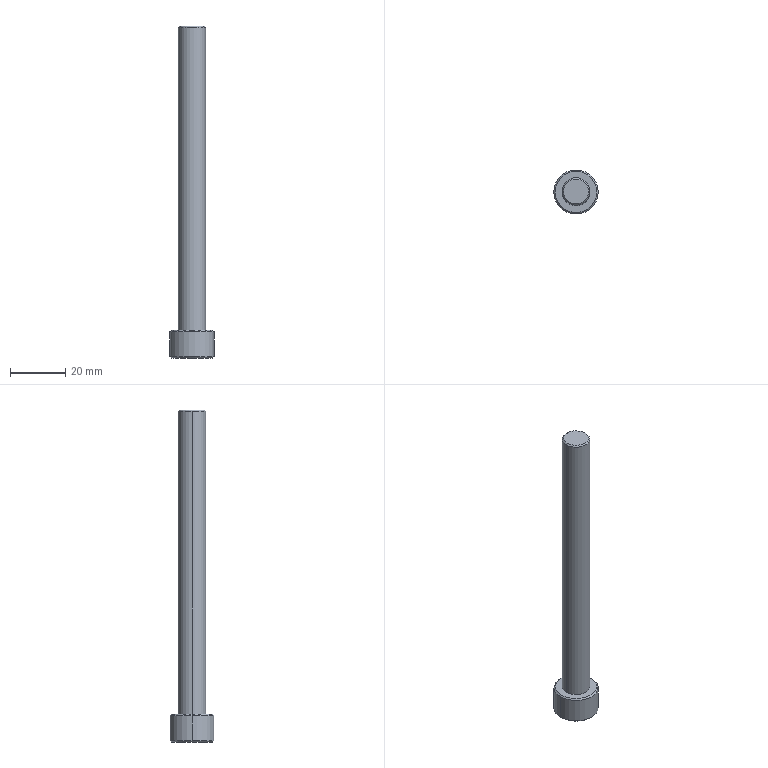Part | SolidWorks | features Chamfer 1, Extrusion 1, ICE 1 | 1 solid | 13 faces | box 16 x 16 x 120 mm | volume 10634 mm3 | cone 6 | cylinder 4 | plane 3 | commonest cylinder face diameters 10 x2 16 x2
STEP:
#1=CARTESIAN_POINT('',(7.5,0.,0.));
#2=VERTEX_POINT('',#1);
#3=CARTESIAN_POINT('',(-7.5,0.,0.));
#4=VERTEX_POINT('',#3);
#5=CARTESIAN_POINT('',(0.,0.,0.));
#6=DIRECTION('',(0.,0.,1.));
#7=DIRECTION('',(-1.,0.,0.));
#8=AXIS2_PLACEMENT_3D('',#5,#6,#7);
#9=CIRCLE('',#8,7.5);
#10=EDGE_CURVE('',#2,#4,#9,.T.);
#11=ORIENTED_EDGE('',*,*,#10,.F.);
#12=CARTESIAN_POINT('',(8.,0.,-0.5));
#13=VERTEX_POINT('',#12);
#14=CARTESIAN_POINT('',(8.,0.,-0.5));
#15=DIRECTION('',(0.7071,0.,-0.7071));
#16=VECTOR('',#15,1000.);
#17=LINE('',#14,#16);
#18=EDGE_CURVE('',#2,#13,#17,.T.);
#19=ORIENTED_EDGE('',*,*,#18,.T.);
#20=CARTESIAN_POINT('',(-8.,0.,-0.5));
#21=VERTEX_POINT('',#20);
#22=CARTESIAN_POINT('',(0.,0.,-0.5));
#23=DIRECTION('',(0.,0.,-1.));
#24=DIRECTION('',(-1.,0.,0.));
#25=AXIS2_PLACEMENT_3D('',#22,#23,#24);
#26=CIRCLE('',#25,8.);
#27=EDGE_CURVE('',#21,#13,#26,.T.);
#28=ORIENTED_EDGE('',*,*,#27,.F.);
#29=CARTESIAN_POINT('',(-8.,0.,-0.5));
#30=DIRECTION('',(-0.7071,0.,-0.7071));
#31=VECTOR('',#30,1000.);
#32=LINE('',#29,#31);
#33=EDGE_CURVE('',#4,#21,#32,.T.);
#34=ORIENTED_EDGE('',*,*,#33,.F.);
#35=EDGE_LOOP('',(#11,#19,#28,#34));
#36=FACE_OUTER_BOUND('',#35,.T.);
#37=CARTESIAN_POINT('',(0.,0.,-0.5));
#38=DIRECTION('',(0.,0.,-1.));
#39=DIRECTION('',(-1.,0.,0.));
#40=AXIS2_PLACEMENT_3D('',#37,#38,#39);
#41=CONICAL_SURFACE('',#40,8.,0.7854);
#42=ADVANCED_FACE('',(#36),#41,.T.);
#43=CARTESIAN_POINT('',(-7.5,0.,-10.));
#44=VERTEX_POINT('',#43);
#45=CARTESIAN_POINT('',(7.5,0.,-10.));
#46=VERTEX_POINT('',#45);
#47=CARTESIAN_POINT('',(0.,0.,-10.));
#48=DIRECTION('',(0.,0.,-1.));
#49=DIRECTION('',(-1.,0.,0.));
#50=AXIS2_PLACEMENT_3D('',#47,#48,#49);
#51=CIRCLE('',#50,7.5);
#52=EDGE_CURVE('',#44,#46,#51,.T.);
#53=ORIENTED_EDGE('',*,*,#52,.F.);
#54=CARTESIAN_POINT('',(-8.,0.,-9.5));
#55=VERTEX_POINT('',#54);
#56=CARTESIAN_POINT('',(-7.5,0.,-10.));
#57=DIRECTION('',(-0.7071,0.,0.7071));
#58=VECTOR('',#57,1000.);
#59=LINE('',#56,#58);
#60=EDGE_CURVE('',#44,#55,#59,.T.);
#61=ORIENTED_EDGE('',*,*,#60,.T.);
#62=CARTESIAN_POINT('',(8.,0.,-9.5));
#63=VERTEX_POINT('',#62);
#64=CARTESIAN_POINT('',(0.,0.,-9.5));
#65=DIRECTION('',(0.,0.,1.));
#66=DIRECTION('',(-1.,0.,0.));
#67=AXIS2_PLACEMENT_3D('',#64,#65,#66);
#68=CIRCLE('',#67,8.);
#69=EDGE_CURVE('',#63,#55,#68,.T.);
#70=ORIENTED_EDGE('',*,*,#69,.F.);
#71=CARTESIAN_POINT('',(7.5,0.,-10.));
#72=DIRECTION('',(0.7071,0.,0.7071));
#73=VECTOR('',#72,1000.);
#74=LINE('',#71,#73);
#75=EDGE_CURVE('',#46,#63,#74,.T.);
#76=ORIENTED_EDGE('',*,*,#75,.F.);
#77=EDGE_LOOP('',(#53,#61,#70,#76));
#78=FACE_OUTER_BOUND('',#77,.T.);
#79=CARTESIAN_POINT('',(0.,0.,-10.));
#80=DIRECTION('',(0.,0.,1.));
#81=DIRECTION('',(1.,0.,0.));
#82=AXIS2_PLACEMENT_3D('',#79,#80,#81);
#83=CONICAL_SURFACE('',#82,7.5,0.7854);
#84=ADVANCED_FACE('',(#78),#83,.T.);
#85=CARTESIAN_POINT('',(4.5,0.,110.));
#86=VERTEX_POINT('',#85);
#87=CARTESIAN_POINT('',(-4.5,0.,110.));
#88=VERTEX_POINT('',#87);
#89=CARTESIAN_POINT('',(0.,0.,110.));
#90=DIRECTION('',(0.,0.,1.));
#91=DIRECTION('',(1.,0.,0.));
#92=AXIS2_PLACEMENT_3D('',#89,#90,#91);
#93=CIRCLE('',#92,4.5);
#94=EDGE_CURVE('',#86,#88,#93,.T.);
#95=ORIENTED_EDGE('',*,*,#94,.F.);
#96=CARTESIAN_POINT('',(5.,0.,109.5));
#97=VERTEX_POINT('',#96);
#98=CARTESIAN_POINT('',(4.5,0.,110.));
#99=DIRECTION('',(0.7071,0.,-0.7071));
#100=VECTOR('',#99,1000.);
#101=LINE('',#98,#100);
#102=EDGE_CURVE('',#86,#97,#101,.T.);
#103=ORIENTED_EDGE('',*,*,#102,.T.);
#104=CARTESIAN_POINT('',(-5.,0.,109.5));
#105=VERTEX_POINT('',#104);
#106=CARTESIAN_POINT('',(0.,0.,109.5));
#107=DIRECTION('',(0.,0.,-1.));
#108=DIRECTION('',(1.,0.,0.));
#109=AXIS2_PLACEMENT_3D('',#106,#107,#108);
#110=CIRCLE('',#109,5.);
#111=EDGE_CURVE('',#105,#97,#110,.T.);
#112=ORIENTED_EDGE('',*,*,#111,.F.);
#113=CARTESIAN_POINT('',(-4.5,0.,110.));
#114=DIRECTION('',(-0.7071,0.,-0.7071));
#115=VECTOR('',#114,1000.);
#116=LINE('',#113,#115);
#117=EDGE_CURVE('',#88,#105,#116,.T.);
#118=ORIENTED_EDGE('',*,*,#117,.F.);
#119=EDGE_LOOP('',(#95,#103,#112,#118));
#120=FACE_OUTER_BOUND('',#119,.T.);
#121=CARTESIAN_POINT('',(0.,0.,110.));
#122=DIRECTION('',(0.,0.,-1.));
#123=DIRECTION('',(-1.,0.,0.));
#124=AXIS2_PLACEMENT_3D('',#121,#122,#123);
#125=CONICAL_SURFACE('',#124,4.5,0.7854);
#126=ADVANCED_FACE('',(#120),#125,.T.);
#127=ORIENTED_EDGE('',*,*,#69,.T.);
#128=CARTESIAN_POINT('',(-8.,0.,-10.));
#129=DIRECTION('',(0.,0.,1.));
#130=VECTOR('',#129,1000.);
#131=LINE('',#128,#130);
#132=EDGE_CURVE('',#55,#21,#131,.T.);
#133=ORIENTED_EDGE('',*,*,#132,.T.);
#134=ORIENTED_EDGE('',*,*,#27,.T.);
#135=CARTESIAN_POINT('',(8.,0.,-10.));
#136=DIRECTION('',(0.,0.,1.));
#137=VECTOR('',#136,1000.);
#138=LINE('',#135,#137);
#139=EDGE_CURVE('',#63,#13,#138,.T.);
#140=ORIENTED_EDGE('',*,*,#139,.F.);
#141=EDGE_LOOP('',(#127,#133,#134,#140));
#142=FACE_OUTER_BOUND('',#141,.T.);
#143=CARTESIAN_POINT('',(0.,0.,-10.));
#144=DIRECTION('',(0.,0.,1.));
#145=DIRECTION('',(1.,0.,0.));
#146=AXIS2_PLACEMENT_3D('',#143,#144,#145);
#147=CYLINDRICAL_SURFACE('',#146,8.);
#148=ADVANCED_FACE('',(#142),#147,.T.);
#149=ORIENTED_EDGE('',*,*,#111,.T.);
#150=CARTESIAN_POINT('',(5.,0.,0.));
#151=VERTEX_POINT('',#150);
#152=CARTESIAN_POINT('',(5.,0.,110.));
#153=DIRECTION('',(0.,0.,-1.));
#154=VECTOR('',#153,1000.);
#155=LINE('',#152,#154);
#156=EDGE_CURVE('',#97,#151,#155,.T.);
#157=ORIENTED_EDGE('',*,*,#156,.T.);
#158=CARTESIAN_POINT('',(-5.,0.,0.));
#159=VERTEX_POINT('',#158);
#160=CARTESIAN_POINT('',(0.,0.,0.));
#161=DIRECTION('',(0.,0.,1.));
#162=DIRECTION('',(1.,0.,0.));
#163=AXIS2_PLACEMENT_3D('',#160,#161,#162);
#164=CIRCLE('',#163,5.);
#165=EDGE_CURVE('',#151,#159,#164,.T.);
#166=ORIENTED_EDGE('',*,*,#165,.T.);
#167=CARTESIAN_POINT('',(-5.,0.,110.));
#168=DIRECTION('',(0.,0.,-1.));
#169=VECTOR('',#168,1000.);
#170=LINE('',#167,#169);
#171=EDGE_CURVE('',#105,#159,#170,.T.);
#172=ORIENTED_EDGE('',*,*,#171,.F.);
#173=EDGE_LOOP('',(#149,#157,#166,#172));
#174=FACE_OUTER_BOUND('',#173,.T.);
#175=CARTESIAN_POINT('',(0.,0.,110.));
#176=DIRECTION('',(0.,0.,-1.));
#177=DIRECTION('',(-1.,0.,0.));
#178=AXIS2_PLACEMENT_3D('',#175,#176,#177);
#179=CYLINDRICAL_SURFACE('',#178,5.);
#180=ADVANCED_FACE('',(#174),#179,.T.);
#181=ORIENTED_EDGE('',*,*,#156,.F.);
#182=CARTESIAN_POINT('',(0.,0.,109.5));
#183=DIRECTION('',(0.,0.,-1.));
#184=DIRECTION('',(1.,0.,0.));
#185=AXIS2_PLACEMENT_3D('',#182,#183,#184);
#186=CIRCLE('',#185,5.);
#187=EDGE_CURVE('',#97,#105,#186,.T.);
#188=ORIENTED_EDGE('',*,*,#187,.T.);
#189=ORIENTED_EDGE('',*,*,#171,.T.);
#190=CARTESIAN_POINT('',(0.,0.,0.));
#191=DIRECTION('',(0.,0.,1.));
#192=DIRECTION('',(1.,0.,0.));
#193=AXIS2_PLACEMENT_3D('',#190,#191,#192);
#194=CIRCLE('',#193,5.);
#195=EDGE_CURVE('',#159,#151,#194,.T.);
#196=ORIENTED_EDGE('',*,*,#195,.T.);
#197=EDGE_LOOP('',(#181,#188,#189,#196));
#198=FACE_OUTER_BOUND('',#197,.T.);
#199=CARTESIAN_POINT('',(0.,0.,110.));
#200=DIRECTION('',(0.,0.,-1.));
#201=DIRECTION('',(-1.,0.,0.));
#202=AXIS2_PLACEMENT_3D('',#199,#200,#201);
#203=CYLINDRICAL_SURFACE('',#202,5.);
#204=ADVANCED_FACE('',(#198),#203,.T.);
#205=CARTESIAN_POINT('',(0.,0.,110.));
#206=DIRECTION('',(0.,0.,1.));
#207=DIRECTION('',(1.,0.,0.));
#208=AXIS2_PLACEMENT_3D('',#205,#206,#207);
#209=CIRCLE('',#208,4.5);
#210=EDGE_CURVE('',#88,#86,#209,.T.);
#211=ORIENTED_EDGE('',*,*,#210,.T.);
#212=ORIENTED_EDGE('',*,*,#94,.T.);
#213=EDGE_LOOP('',(#211,#212));
#214=FACE_OUTER_BOUND('',#213,.T.);
#215=CARTESIAN_POINT('',(0.,0.,110.));
#216=DIRECTION('',(0.,0.,1.));
#217=DIRECTION('',(1.,0.,0.));
#218=AXIS2_PLACEMENT_3D('',#215,#216,#217);
#219=PLANE('',#218);
#220=ADVANCED_FACE('',(#214),#219,.T.);
#221=ORIENTED_EDGE('',*,*,#132,.F.);
#222=CARTESIAN_POINT('',(0.,0.,-9.5));
#223=DIRECTION('',(0.,0.,1.));
#224=DIRECTION('',(-1.,0.,0.));
#225=AXIS2_PLACEMENT_3D('',#222,#223,#224);
#226=CIRCLE('',#225,8.);
#227=EDGE_CURVE('',#55,#63,#226,.T.);
#228=ORIENTED_EDGE('',*,*,#227,.T.);
#229=ORIENTED_EDGE('',*,*,#139,.T.);
#230=CARTESIAN_POINT('',(0.,0.,-0.5));
#231=DIRECTION('',(0.,0.,-1.));
#232=DIRECTION('',(-1.,0.,0.));
#233=AXIS2_PLACEMENT_3D('',#230,#231,#232);
#234=CIRCLE('',#233,8.);
#235=EDGE_CURVE('',#13,#21,#234,.T.);
#236=ORIENTED_EDGE('',*,*,#235,.T.);
#237=EDGE_LOOP('',(#221,#228,#229,#236));
#238=FACE_OUTER_BOUND('',#237,.T.);
#239=CARTESIAN_POINT('',(0.,0.,-10.));
#240=DIRECTION('',(0.,0.,1.));
#241=DIRECTION('',(1.,0.,0.));
#242=AXIS2_PLACEMENT_3D('',#239,#240,#241);
#243=CYLINDRICAL_SURFACE('',#242,8.);
#244=ADVANCED_FACE('',(#238),#243,.T.);
#245=CARTESIAN_POINT('',(0.,0.,-10.));
#246=DIRECTION('',(0.,0.,-1.));
#247=DIRECTION('',(-1.,0.,0.));
#248=AXIS2_PLACEMENT_3D('',#245,#246,#247);
#249=CIRCLE('',#248,7.5);
#250=EDGE_CURVE('',#46,#44,#249,.T.);
#251=ORIENTED_EDGE('',*,*,#250,.T.);
#252=ORIENTED_EDGE('',*,*,#52,.T.);
#253=EDGE_LOOP('',(#251,#252));
#254=FACE_OUTER_BOUND('',#253,.T.);
#255=CARTESIAN_POINT('',(0.,0.,-10.));
#256=DIRECTION('',(0.,0.,-1.));
#257=DIRECTION('',(-1.,0.,0.));
#258=AXIS2_PLACEMENT_3D('',#255,#256,#257);
#259=PLANE('',#258);
#260=ADVANCED_FACE('',(#254),#259,.T.);
#261=CARTESIAN_POINT('',(0.,0.,0.));
#262=DIRECTION('',(0.,0.,1.));
#263=DIRECTION('',(-1.,0.,0.));
#264=AXIS2_PLACEMENT_3D('',#261,#262,#263);
#265=CIRCLE('',#264,7.5);
#266=EDGE_CURVE('',#4,#2,#265,.T.);
#267=ORIENTED_EDGE('',*,*,#266,.T.);
#268=ORIENTED_EDGE('',*,*,#10,.T.);
#269=EDGE_LOOP('',(#267,#268));
#270=FACE_OUTER_BOUND('',#269,.T.);
#271=ORIENTED_EDGE('',*,*,#195,.F.);
#272=ORIENTED_EDGE('',*,*,#165,.F.);
#273=EDGE_LOOP('',(#271,#272));
#274=FACE_BOUND('',#273,.T.);
#275=CARTESIAN_POINT('',(0.,0.,0.));
#276=DIRECTION('',(0.,0.,-1.));
#277=DIRECTION('',(-1.,0.,0.));
#278=AXIS2_PLACEMENT_3D('',#275,#276,#277);
#279=PLANE('',#278);
#280=ADVANCED_FACE('',(#270,#274),#279,.F.);
#281=ORIENTED_EDGE('',*,*,#102,.F.);
#282=ORIENTED_EDGE('',*,*,#210,.F.);
#283=ORIENTED_EDGE('',*,*,#117,.T.);
#284=ORIENTED_EDGE('',*,*,#187,.F.);
#285=EDGE_LOOP('',(#281,#282,#283,#284));
#286=FACE_OUTER_BOUND('',#285,.T.);
#287=CARTESIAN_POINT('',(0.,0.,110.));
#288=DIRECTION('',(0.,0.,-1.));
#289=DIRECTION('',(-1.,0.,0.));
#290=AXIS2_PLACEMENT_3D('',#287,#288,#289);
#291=CONICAL_SURFACE('',#290,4.5,0.7854);
#292=ADVANCED_FACE('',(#286),#291,.T.);
#293=ORIENTED_EDGE('',*,*,#60,.F.);
#294=ORIENTED_EDGE('',*,*,#250,.F.);
#295=ORIENTED_EDGE('',*,*,#75,.T.);
#296=ORIENTED_EDGE('',*,*,#227,.F.);
#297=EDGE_LOOP('',(#293,#294,#295,#296));
#298=FACE_OUTER_BOUND('',#297,.T.);
#299=CARTESIAN_POINT('',(0.,0.,-10.));
#300=DIRECTION('',(0.,0.,1.));
#301=DIRECTION('',(1.,0.,0.));
#302=AXIS2_PLACEMENT_3D('',#299,#300,#301);
#303=CONICAL_SURFACE('',#302,7.5,0.7854);
#304=ADVANCED_FACE('',(#298),#303,.T.);
#305=ORIENTED_EDGE('',*,*,#18,.F.);
#306=ORIENTED_EDGE('',*,*,#266,.F.);
#307=ORIENTED_EDGE('',*,*,#33,.T.);
#308=ORIENTED_EDGE('',*,*,#235,.F.);
#309=EDGE_LOOP('',(#305,#306,#307,#308));
#310=FACE_OUTER_BOUND('',#309,.T.);
#311=CARTESIAN_POINT('',(0.,0.,-0.5));
#312=DIRECTION('',(0.,0.,-1.));
#313=DIRECTION('',(-1.,0.,0.));
#314=AXIS2_PLACEMENT_3D('',#311,#312,#313);
#315=CONICAL_SURFACE('',#314,8.,0.7854);
#316=ADVANCED_FACE('',(#310),#315,.T.);
#317=CLOSED_SHELL('',(#42,#84,#126,#148,#180,#204,#220,#244,#260,#280,#292,#304,#316));
#318=MANIFOLD_SOLID_BREP('',#317);
#319=CARTESIAN_POINT('',(0.,0.,0.));
#320=DIRECTION('',(0.,0.,1.));
#321=DIRECTION('',(1.,0.,0.));
#322=AXIS2_PLACEMENT_3D('',#319,#320,#321);
#323=(LENGTH_UNIT()NAMED_UNIT(*)SI_UNIT(.MILLI.,.METRE.));
#324=UNCERTAINTY_MEASURE_WITH_UNIT(LENGTH_MEASURE(0.00001),#323,'','');
#325=(NAMED_UNIT(*)PLANE_ANGLE_UNIT()SI_UNIT($,.RADIAN.));
#326=(NAMED_UNIT(*)SI_UNIT($,.STERADIAN.)SOLID_ANGLE_UNIT());
#327=(GEOMETRIC_REPRESENTATION_CONTEXT(3)GLOBAL_UNCERTAINTY_ASSIGNED_CONTEXT((#324))GLOBAL_UNIT_ASSIGNED_CONTEXT((#323,#325,#326))REPRESENTATION_CONTEXT('',''));
#328=ADVANCED_BREP_SHAPE_REPRESENTATION('',(#318,#322),#327);